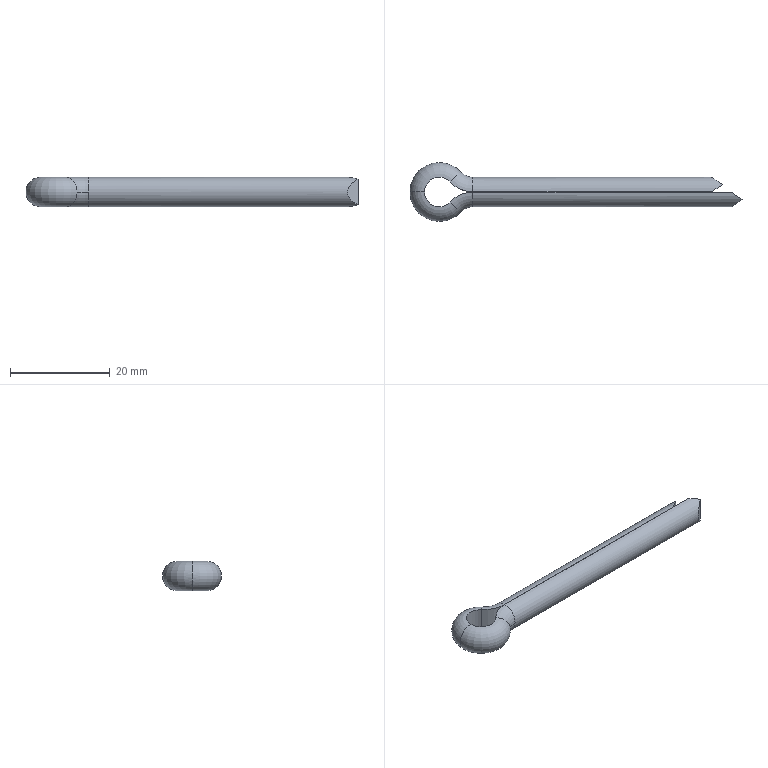Part | SolidWorks | features ICE 1, Sweep 1 | 1 solid | 18 faces | box 66.6 x 11.8 x 5.9 mm | volume 1774 mm3 | torus 6 | cylinder 6 | plane 6 | commonest cylinder face diameters 5.9 x3 12.247 x2 5.92 x1
STEP:
#1=CARTESIAN_POINT('',(6.7,0.01,2.95));
#2=VERTEX_POINT('',#1);
#3=CARTESIAN_POINT('',(6.7,2.95,0.));
#4=VERTEX_POINT('',#3);
#5=CARTESIAN_POINT('',(6.7,0.,0.));
#6=DIRECTION('',(-1.,0.,0.));
#7=DIRECTION('',(0.,0.,1.));
#8=AXIS2_PLACEMENT_3D('',#5,#6,#7);
#9=CIRCLE('',#8,2.95);
#10=EDGE_CURVE('',#2,#4,#9,.T.);
#11=ORIENTED_EDGE('',*,*,#10,.T.);
#12=CARTESIAN_POINT('',(4.352,3.984,0.));
#13=VERTEX_POINT('',#12);
#14=CARTESIAN_POINT('',(6.7,6.133,0.));
#15=DIRECTION('',(0.,0.,-1.));
#16=DIRECTION('',(-1.,0.,0.));
#17=AXIS2_PLACEMENT_3D('',#14,#15,#16);
#18=CIRCLE('',#17,3.183);
#19=EDGE_CURVE('',#4,#13,#18,.T.);
#20=ORIENTED_EDGE('',*,*,#19,.T.);
#21=CARTESIAN_POINT('',(2.183,1.999,2.95));
#22=VERTEX_POINT('',#21);
#23=CARTESIAN_POINT('',(2.176,1.992,0.));
#24=DIRECTION('',(-0.6752,0.7376,0.));
#25=DIRECTION('',(0.,0.,1.));
#26=AXIS2_PLACEMENT_3D('',#23,#24,#25);
#27=CIRCLE('',#26,2.95);
#28=EDGE_CURVE('',#22,#13,#27,.T.);
#29=ORIENTED_EDGE('',*,*,#28,.F.);
#30=CARTESIAN_POINT('',(6.7,6.133,2.95));
#31=DIRECTION('',(0.,0.,-1.));
#32=DIRECTION('',(-1.,0.,0.));
#33=AXIS2_PLACEMENT_3D('',#30,#31,#32);
#34=CIRCLE('',#33,6.123);
#35=EDGE_CURVE('',#2,#22,#34,.T.);
#36=ORIENTED_EDGE('',*,*,#35,.F.);
#37=EDGE_LOOP('',(#11,#20,#29,#36));
#38=FACE_OUTER_BOUND('',#37,.T.);
#39=CARTESIAN_POINT('',(6.7,6.133,0.));
#40=DIRECTION('',(0.,0.,-1.));
#41=DIRECTION('',(-1.,0.,0.));
#42=AXIS2_PLACEMENT_3D('',#39,#40,#41);
#43=TOROIDAL_SURFACE('',#42,6.133,2.95);
#44=ADVANCED_FACE('',(#38),#43,.T.);
#45=CARTESIAN_POINT('',(2.183,-1.999,2.95));
#46=VERTEX_POINT('',#45);
#47=CARTESIAN_POINT('',(4.352,-3.984,0.));
#48=VERTEX_POINT('',#47);
#49=CARTESIAN_POINT('',(2.176,-1.992,0.));
#50=DIRECTION('',(0.6752,0.7376,0.));
#51=DIRECTION('',(0.,0.,1.));
#52=AXIS2_PLACEMENT_3D('',#49,#50,#51);
#53=CIRCLE('',#52,2.95);
#54=EDGE_CURVE('',#46,#48,#53,.T.);
#55=ORIENTED_EDGE('',*,*,#54,.T.);
#56=CARTESIAN_POINT('',(6.7,-2.95,0.));
#57=VERTEX_POINT('',#56);
#58=CARTESIAN_POINT('',(6.7,-6.133,0.));
#59=DIRECTION('',(0.,0.,-1.));
#60=DIRECTION('',(-1.,0.,0.));
#61=AXIS2_PLACEMENT_3D('',#58,#59,#60);
#62=CIRCLE('',#61,3.183);
#63=EDGE_CURVE('',#48,#57,#62,.T.);
#64=ORIENTED_EDGE('',*,*,#63,.T.);
#65=CARTESIAN_POINT('',(6.7,-0.01,2.95));
#66=VERTEX_POINT('',#65);
#67=CARTESIAN_POINT('',(6.7,0.,0.));
#68=DIRECTION('',(1.,0.,0.));
#69=DIRECTION('',(0.,0.,1.));
#70=AXIS2_PLACEMENT_3D('',#67,#68,#69);
#71=CIRCLE('',#70,2.95);
#72=EDGE_CURVE('',#66,#57,#71,.T.);
#73=ORIENTED_EDGE('',*,*,#72,.F.);
#74=CARTESIAN_POINT('',(6.7,-6.133,2.95));
#75=DIRECTION('',(0.,0.,-1.));
#76=DIRECTION('',(-1.,0.,0.));
#77=AXIS2_PLACEMENT_3D('',#74,#75,#76);
#78=CIRCLE('',#77,6.123);
#79=EDGE_CURVE('',#46,#66,#78,.T.);
#80=ORIENTED_EDGE('',*,*,#79,.F.);
#81=EDGE_LOOP('',(#55,#64,#73,#80));
#82=FACE_OUTER_BOUND('',#81,.T.);
#83=CARTESIAN_POINT('',(6.7,-6.133,0.));
#84=DIRECTION('',(0.,0.,-1.));
#85=DIRECTION('',(-1.,0.,0.));
#86=AXIS2_PLACEMENT_3D('',#83,#84,#85);
#87=TOROIDAL_SURFACE('',#86,6.133,2.95);
#88=ADVANCED_FACE('',(#82),#87,.T.);
#89=CARTESIAN_POINT('',(6.7,0.01,-2.95));
#90=VERTEX_POINT('',#89);
#91=CARTESIAN_POINT('',(6.7,0.,0.));
#92=DIRECTION('',(-1.,0.,0.));
#93=DIRECTION('',(0.,0.,1.));
#94=AXIS2_PLACEMENT_3D('',#91,#92,#93);
#95=CIRCLE('',#94,2.95);
#96=EDGE_CURVE('',#4,#90,#95,.T.);
#97=ORIENTED_EDGE('',*,*,#96,.F.);
#98=CARTESIAN_POINT('',(54.597,2.95,0.));
#99=VERTEX_POINT('',#98);
#100=CARTESIAN_POINT('',(6.7,2.95,0.));
#101=DIRECTION('',(1.,0.,0.));
#102=VECTOR('',#101,1000.);
#103=LINE('',#100,#102);
#104=EDGE_CURVE('',#4,#99,#103,.T.);
#105=ORIENTED_EDGE('',*,*,#104,.T.);
#106=CARTESIAN_POINT('',(56.7,1.47,-2.558));
#107=VERTEX_POINT('',#106);
#108=CARTESIAN_POINT('',(54.597,2.95,0.));
#109=CARTESIAN_POINT('',(54.597,2.95,-1.082));
#110=CARTESIAN_POINT('',(55.367,2.408,-2.018));
#111=CARTESIAN_POINT('',(56.7,1.47,-2.558));
#112=(BOUNDED_CURVE()B_SPLINE_CURVE(3,(#108,#109,#110,#111),.UNSPECIFIED.,.F.,.T.)B_SPLINE_CURVE_WITH_KNOTS((4,4),(3.142,4.191),.UNSPECIFIED.)CURVE()GEOMETRIC_REPRESENTATION_ITEM()RATIONAL_B_SPLINE_CURVE((1.,0.9104,0.9104,1.))REPRESENTATION_ITEM(''));
#113=EDGE_CURVE('',#99,#107,#112,.T.);
#114=ORIENTED_EDGE('',*,*,#113,.T.);
#115=CARTESIAN_POINT('',(54.604,0.01,-2.95));
#116=VERTEX_POINT('',#115);
#117=CARTESIAN_POINT('',(56.7,1.47,-2.558));
#118=CARTESIAN_POINT('',(56.059,1.023,-2.814));
#119=CARTESIAN_POINT('',(55.344,0.5254,-2.948));
#120=CARTESIAN_POINT('',(54.604,0.01,-2.95));
#121=(BOUNDED_CURVE()B_SPLINE_CURVE(3,(#117,#118,#119,#120),.UNSPECIFIED.,.F.,.T.)B_SPLINE_CURVE_WITH_KNOTS((4,4),(1.049,1.567),.UNSPECIFIED.)CURVE()GEOMETRIC_REPRESENTATION_ITEM()RATIONAL_B_SPLINE_CURVE((1.,0.9777,0.9777,1.))REPRESENTATION_ITEM(''));
#122=EDGE_CURVE('',#107,#116,#121,.T.);
#123=ORIENTED_EDGE('',*,*,#122,.T.);
#124=CARTESIAN_POINT('',(6.7,0.01,-2.95));
#125=DIRECTION('',(1.,0.,0.));
#126=VECTOR('',#125,1000.);
#127=LINE('',#124,#126);
#128=EDGE_CURVE('',#90,#116,#127,.T.);
#129=ORIENTED_EDGE('',*,*,#128,.F.);
#130=EDGE_LOOP('',(#97,#105,#114,#123,#129));
#131=FACE_OUTER_BOUND('',#130,.T.);
#132=CARTESIAN_POINT('',(6.7,0.,0.));
#133=DIRECTION('',(1.,0.,0.));
#134=DIRECTION('',(0.,1.,0.));
#135=AXIS2_PLACEMENT_3D('',#132,#133,#134);
#136=CYLINDRICAL_SURFACE('',#135,2.95);
#137=ADVANCED_FACE('',(#131),#136,.T.);
#138=CARTESIAN_POINT('',(2.183,1.999,-2.95));
#139=VERTEX_POINT('',#138);
#140=CARTESIAN_POINT('',(-2.96,0.,-2.95));
#141=VERTEX_POINT('',#140);
#142=CARTESIAN_POINT('',(0.,0.,-2.95));
#143=DIRECTION('',(0.,0.,1.));
#144=DIRECTION('',(1.,0.,0.));
#145=AXIS2_PLACEMENT_3D('',#142,#143,#144);
#146=CIRCLE('',#145,2.96);
#147=EDGE_CURVE('',#139,#141,#146,.T.);
#148=ORIENTED_EDGE('',*,*,#147,.T.);
#149=CARTESIAN_POINT('',(-2.96,0.,2.95));
#150=VERTEX_POINT('',#149);
#151=CARTESIAN_POINT('',(-2.95,0.,0.));
#152=DIRECTION('',(0.,1.,0.));
#153=DIRECTION('',(-1.,0.,0.));
#154=AXIS2_PLACEMENT_3D('',#151,#152,#153);
#155=CIRCLE('',#154,2.95);
#156=EDGE_CURVE('',#141,#150,#155,.T.);
#157=ORIENTED_EDGE('',*,*,#156,.T.);
#158=CARTESIAN_POINT('',(0.,0.,2.95));
#159=DIRECTION('',(0.,0.,1.));
#160=DIRECTION('',(1.,0.,0.));
#161=AXIS2_PLACEMENT_3D('',#158,#159,#160);
#162=CIRCLE('',#161,2.96);
#163=EDGE_CURVE('',#22,#150,#162,.T.);
#164=ORIENTED_EDGE('',*,*,#163,.F.);
#165=ORIENTED_EDGE('',*,*,#28,.T.);
#166=CARTESIAN_POINT('',(2.176,1.992,0.));
#167=DIRECTION('',(-0.6752,0.7376,0.));
#168=DIRECTION('',(0.,0.,1.));
#169=AXIS2_PLACEMENT_3D('',#166,#167,#168);
#170=CIRCLE('',#169,2.95);
#171=EDGE_CURVE('',#13,#139,#170,.T.);
#172=ORIENTED_EDGE('',*,*,#171,.T.);
#173=EDGE_LOOP('',(#148,#157,#164,#165,#172));
#174=FACE_OUTER_BOUND('',#173,.T.);
#175=CARTESIAN_POINT('',(0.,0.,0.));
#176=DIRECTION('',(0.,0.,1.));
#177=DIRECTION('',(1.,0.,0.));
#178=AXIS2_PLACEMENT_3D('',#175,#176,#177);
#179=TOROIDAL_SURFACE('',#178,2.95,2.95);
#180=ADVANCED_FACE('',(#174),#179,.T.);
#181=CARTESIAN_POINT('',(60.7,-1.48,-2.552));
#182=VERTEX_POINT('',#181);
#183=CARTESIAN_POINT('',(58.611,-0.01,-2.95));
#184=VERTEX_POINT('',#183);
#185=CARTESIAN_POINT('',(60.7,-1.48,-2.552));
#186=CARTESIAN_POINT('',(60.062,-1.031,-2.812));
#187=CARTESIAN_POINT('',(59.349,-0.5294,-2.948));
#188=CARTESIAN_POINT('',(58.611,-0.01,-2.95));
#189=(BOUNDED_CURVE()B_SPLINE_CURVE(3,(#185,#186,#187,#188),.UNSPECIFIED.,.F.,.F.)B_SPLINE_CURVE_WITH_KNOTS((4,4),(1.045,1.567),.UNSPECIFIED.)CURVE()GEOMETRIC_REPRESENTATION_ITEM()RATIONAL_B_SPLINE_CURVE((1.,0.9774,0.9774,1.))REPRESENTATION_ITEM(''));
#190=EDGE_CURVE('',#182,#184,#189,.T.);
#191=ORIENTED_EDGE('',*,*,#190,.F.);
#192=CARTESIAN_POINT('',(60.7,-1.48,2.552));
#193=VERTEX_POINT('',#192);
#194=CARTESIAN_POINT('',(60.7,-1.48,2.552));
#195=CARTESIAN_POINT('',(57.537,-3.684,1.274));
#196=CARTESIAN_POINT('',(57.537,-3.684,-1.274));
#197=CARTESIAN_POINT('',(60.7,-1.48,-2.552));
#198=(BOUNDED_CURVE()B_SPLINE_CURVE(3,(#194,#195,#196,#197),.UNSPECIFIED.,.F.,.T.)B_SPLINE_CURVE_WITH_KNOTS((4,4),(2.096,4.187),.UNSPECIFIED.)CURVE()GEOMETRIC_REPRESENTATION_ITEM()RATIONAL_B_SPLINE_CURVE((1.,0.6678,0.6678,1.))REPRESENTATION_ITEM(''));
#199=EDGE_CURVE('',#193,#182,#198,.T.);
#200=ORIENTED_EDGE('',*,*,#199,.F.);
#201=CARTESIAN_POINT('',(58.611,-0.01,2.95));
#202=VERTEX_POINT('',#201);
#203=CARTESIAN_POINT('',(58.611,-0.01,2.95));
#204=CARTESIAN_POINT('',(59.349,-0.5294,2.948));
#205=CARTESIAN_POINT('',(60.062,-1.031,2.812));
#206=CARTESIAN_POINT('',(60.7,-1.48,2.552));
#207=(BOUNDED_CURVE()B_SPLINE_CURVE(3,(#203,#204,#205,#206),.UNSPECIFIED.,.F.,.F.)B_SPLINE_CURVE_WITH_KNOTS((4,4),(4.716,5.238),.UNSPECIFIED.)CURVE()GEOMETRIC_REPRESENTATION_ITEM()RATIONAL_B_SPLINE_CURVE((1.,0.9774,0.9774,1.))REPRESENTATION_ITEM(''));
#208=EDGE_CURVE('',#202,#193,#207,.T.);
#209=ORIENTED_EDGE('',*,*,#208,.F.);
#210=CARTESIAN_POINT('',(6.7,-0.01,2.95));
#211=DIRECTION('',(1.,0.,0.));
#212=VECTOR('',#211,1000.);
#213=LINE('',#210,#212);
#214=EDGE_CURVE('',#66,#202,#213,.T.);
#215=ORIENTED_EDGE('',*,*,#214,.F.);
#216=ORIENTED_EDGE('',*,*,#72,.T.);
#217=CARTESIAN_POINT('',(6.7,-0.01,-2.95));
#218=VERTEX_POINT('',#217);
#219=CARTESIAN_POINT('',(6.7,0.,0.));
#220=DIRECTION('',(1.,0.,0.));
#221=DIRECTION('',(0.,0.,1.));
#222=AXIS2_PLACEMENT_3D('',#219,#220,#221);
#223=CIRCLE('',#222,2.95);
#224=EDGE_CURVE('',#57,#218,#223,.T.);
#225=ORIENTED_EDGE('',*,*,#224,.T.);
#226=CARTESIAN_POINT('',(6.7,-0.01,-2.95));
#227=DIRECTION('',(1.,0.,0.));
#228=VECTOR('',#227,1000.);
#229=LINE('',#226,#228);
#230=EDGE_CURVE('',#218,#184,#229,.T.);
#231=ORIENTED_EDGE('',*,*,#230,.T.);
#232=EDGE_LOOP('',(#191,#200,#209,#215,#216,#225,#231));
#233=FACE_OUTER_BOUND('',#232,.T.);
#234=CARTESIAN_POINT('',(6.7,0.,0.));
#235=DIRECTION('',(1.,0.,0.));
#236=DIRECTION('',(0.,1.,0.));
#237=AXIS2_PLACEMENT_3D('',#234,#235,#236);
#238=CYLINDRICAL_SURFACE('',#237,2.95);
#239=ADVANCED_FACE('',(#233),#238,.T.);
#240=CARTESIAN_POINT('',(58.611,-0.01,-2.95));
#241=DIRECTION('',(0.,0.,1.));
#242=VECTOR('',#241,1000.);
#243=LINE('',#240,#242);
#244=EDGE_CURVE('',#184,#202,#243,.T.);
#245=ORIENTED_EDGE('',*,*,#244,.F.);
#246=ORIENTED_EDGE('',*,*,#230,.F.);
#247=CARTESIAN_POINT('',(6.7,-0.01,-2.95));
#248=DIRECTION('',(0.,0.,1.));
#249=VECTOR('',#248,1000.);
#250=LINE('',#247,#249);
#251=EDGE_CURVE('',#218,#66,#250,.T.);
#252=ORIENTED_EDGE('',*,*,#251,.T.);
#253=ORIENTED_EDGE('',*,*,#214,.T.);
#254=EDGE_LOOP('',(#245,#246,#252,#253));
#255=FACE_OUTER_BOUND('',#254,.T.);
#256=CARTESIAN_POINT('',(6.7,-0.01,-2.95));
#257=DIRECTION('',(0.,1.,0.));
#258=DIRECTION('',(-1.,0.,0.));
#259=AXIS2_PLACEMENT_3D('',#256,#257,#258);
#260=PLANE('',#259);
#261=ADVANCED_FACE('',(#255),#260,.T.);
#262=CARTESIAN_POINT('',(2.183,-1.999,-2.95));
#263=VERTEX_POINT('',#262);
#264=CARTESIAN_POINT('',(2.183,-1.999,-2.95));
#265=DIRECTION('',(0.,0.,1.));
#266=VECTOR('',#265,1000.);
#267=LINE('',#264,#266);
#268=EDGE_CURVE('',#263,#46,#267,.T.);
#269=ORIENTED_EDGE('',*,*,#268,.T.);
#270=ORIENTED_EDGE('',*,*,#79,.T.);
#271=ORIENTED_EDGE('',*,*,#251,.F.);
#272=CARTESIAN_POINT('',(6.7,-6.133,-2.95));
#273=DIRECTION('',(0.,0.,-1.));
#274=DIRECTION('',(-1.,0.,0.));
#275=AXIS2_PLACEMENT_3D('',#272,#273,#274);
#276=CIRCLE('',#275,6.123);
#277=EDGE_CURVE('',#263,#218,#276,.T.);
#278=ORIENTED_EDGE('',*,*,#277,.F.);
#279=EDGE_LOOP('',(#269,#270,#271,#278));
#280=FACE_OUTER_BOUND('',#279,.T.);
#281=CARTESIAN_POINT('',(6.7,-6.133,0.));
#282=DIRECTION('',(0.,0.,-1.));
#283=DIRECTION('',(-1.,0.,0.));
#284=AXIS2_PLACEMENT_3D('',#281,#282,#283);
#285=CYLINDRICAL_SURFACE('',#284,6.123);
#286=ADVANCED_FACE('',(#280),#285,.T.);
#287=ORIENTED_EDGE('',*,*,#63,.F.);
#288=CARTESIAN_POINT('',(2.176,-1.992,0.));
#289=DIRECTION('',(0.6752,0.7376,0.));
#290=DIRECTION('',(0.,0.,1.));
#291=AXIS2_PLACEMENT_3D('',#288,#289,#290);
#292=CIRCLE('',#291,2.95);
#293=EDGE_CURVE('',#48,#263,#292,.T.);
#294=ORIENTED_EDGE('',*,*,#293,.T.);
#295=ORIENTED_EDGE('',*,*,#277,.T.);
#296=ORIENTED_EDGE('',*,*,#224,.F.);
#297=EDGE_LOOP('',(#287,#294,#295,#296));
#298=FACE_OUTER_BOUND('',#297,.T.);
#299=CARTESIAN_POINT('',(6.7,-6.133,0.));
#300=DIRECTION('',(0.,0.,-1.));
#301=DIRECTION('',(-1.,0.,0.));
#302=AXIS2_PLACEMENT_3D('',#299,#300,#301);
#303=TOROIDAL_SURFACE('',#302,6.133,2.95);
#304=ADVANCED_FACE('',(#298),#303,.T.);
#305=CARTESIAN_POINT('',(2.183,1.999,-2.95));
#306=DIRECTION('',(0.,0.,1.));
#307=VECTOR('',#306,1000.);
#308=LINE('',#305,#307);
#309=EDGE_CURVE('',#139,#22,#308,.T.);
#310=ORIENTED_EDGE('',*,*,#309,.T.);
#311=ORIENTED_EDGE('',*,*,#163,.T.);
#312=CARTESIAN_POINT('',(0.,0.,2.95));
#313=DIRECTION('',(0.,0.,1.));
#314=DIRECTION('',(1.,0.,0.));
#315=AXIS2_PLACEMENT_3D('',#312,#313,#314);
#316=CIRCLE('',#315,2.96);
#317=EDGE_CURVE('',#150,#46,#316,.T.);
#318=ORIENTED_EDGE('',*,*,#317,.T.);
#319=ORIENTED_EDGE('',*,*,#268,.F.);
#320=CARTESIAN_POINT('',(0.,0.,-2.95));
#321=DIRECTION('',(0.,0.,1.));
#322=DIRECTION('',(1.,0.,0.));
#323=AXIS2_PLACEMENT_3D('',#320,#321,#322);
#324=CIRCLE('',#323,2.96);
#325=EDGE_CURVE('',#141,#263,#324,.T.);
#326=ORIENTED_EDGE('',*,*,#325,.F.);
#327=ORIENTED_EDGE('',*,*,#147,.F.);
#328=EDGE_LOOP('',(#310,#311,#318,#319,#326,#327));
#329=FACE_OUTER_BOUND('',#328,.T.);
#330=CARTESIAN_POINT('',(0.,0.,0.));
#331=DIRECTION('',(0.,0.,1.));
#332=DIRECTION('',(1.,0.,0.));
#333=AXIS2_PLACEMENT_3D('',#330,#331,#332);
#334=CYLINDRICAL_SURFACE('',#333,2.96);
#335=ADVANCED_FACE('',(#329),#334,.F.);
#336=ORIENTED_EDGE('',*,*,#156,.F.);
#337=ORIENTED_EDGE('',*,*,#325,.T.);
#338=ORIENTED_EDGE('',*,*,#293,.F.);
#339=ORIENTED_EDGE('',*,*,#54,.F.);
#340=ORIENTED_EDGE('',*,*,#317,.F.);
#341=EDGE_LOOP('',(#336,#337,#338,#339,#340));
#342=FACE_OUTER_BOUND('',#341,.T.);
#343=CARTESIAN_POINT('',(0.,0.,0.));
#344=DIRECTION('',(0.,0.,1.));
#345=DIRECTION('',(1.,0.,0.));
#346=AXIS2_PLACEMENT_3D('',#343,#344,#345);
#347=TOROIDAL_SURFACE('',#346,2.95,2.95);
#348=ADVANCED_FACE('',(#342),#347,.T.);
#349=CARTESIAN_POINT('',(6.7,0.01,-2.95));
#350=DIRECTION('',(0.,0.,1.));
#351=VECTOR('',#350,1000.);
#352=LINE('',#349,#351);
#353=EDGE_CURVE('',#90,#2,#352,.T.);
#354=ORIENTED_EDGE('',*,*,#353,.T.);
#355=ORIENTED_EDGE('',*,*,#35,.T.);
#356=ORIENTED_EDGE('',*,*,#309,.F.);
#357=CARTESIAN_POINT('',(6.7,6.133,-2.95));
#358=DIRECTION('',(0.,0.,-1.));
#359=DIRECTION('',(-1.,0.,0.));
#360=AXIS2_PLACEMENT_3D('',#357,#358,#359);
#361=CIRCLE('',#360,6.123);
#362=EDGE_CURVE('',#90,#139,#361,.T.);
#363=ORIENTED_EDGE('',*,*,#362,.F.);
#364=EDGE_LOOP('',(#354,#355,#356,#363));
#365=FACE_OUTER_BOUND('',#364,.T.);
#366=CARTESIAN_POINT('',(6.7,6.133,0.));
#367=DIRECTION('',(0.,0.,-1.));
#368=DIRECTION('',(-1.,0.,0.));
#369=AXIS2_PLACEMENT_3D('',#366,#367,#368);
#370=CYLINDRICAL_SURFACE('',#369,6.123);
#371=ADVANCED_FACE('',(#365),#370,.T.);
#372=ORIENTED_EDGE('',*,*,#19,.F.);
#373=ORIENTED_EDGE('',*,*,#96,.T.);
#374=ORIENTED_EDGE('',*,*,#362,.T.);
#375=ORIENTED_EDGE('',*,*,#171,.F.);
#376=EDGE_LOOP('',(#372,#373,#374,#375));
#377=FACE_OUTER_BOUND('',#376,.T.);
#378=CARTESIAN_POINT('',(6.7,6.133,0.));
#379=DIRECTION('',(0.,0.,-1.));
#380=DIRECTION('',(-1.,0.,0.));
#381=AXIS2_PLACEMENT_3D('',#378,#379,#380);
#382=TOROIDAL_SURFACE('',#381,6.133,2.95);
#383=ADVANCED_FACE('',(#377),#382,.T.);
#384=ORIENTED_EDGE('',*,*,#104,.F.);
#385=ORIENTED_EDGE('',*,*,#10,.F.);
#386=CARTESIAN_POINT('',(54.604,0.01,2.95));
#387=VERTEX_POINT('',#386);
#388=CARTESIAN_POINT('',(6.7,0.01,2.95));
#389=DIRECTION('',(1.,0.,0.));
#390=VECTOR('',#389,1000.);
#391=LINE('',#388,#390);
#392=EDGE_CURVE('',#2,#387,#391,.T.);
#393=ORIENTED_EDGE('',*,*,#392,.T.);
#394=CARTESIAN_POINT('',(56.7,1.47,2.558));
#395=VERTEX_POINT('',#394);
#396=CARTESIAN_POINT('',(54.604,0.01,2.95));
#397=CARTESIAN_POINT('',(55.344,0.5254,2.948));
#398=CARTESIAN_POINT('',(56.059,1.023,2.814));
#399=CARTESIAN_POINT('',(56.7,1.47,2.558));
#400=(BOUNDED_CURVE()B_SPLINE_CURVE(3,(#396,#397,#398,#399),.UNSPECIFIED.,.F.,.F.)B_SPLINE_CURVE_WITH_KNOTS((4,4),(4.716,5.234),.UNSPECIFIED.)CURVE()GEOMETRIC_REPRESENTATION_ITEM()RATIONAL_B_SPLINE_CURVE((1.,0.9777,0.9777,1.))REPRESENTATION_ITEM(''));
#401=EDGE_CURVE('',#387,#395,#400,.T.);
#402=ORIENTED_EDGE('',*,*,#401,.T.);
#403=CARTESIAN_POINT('',(56.7,1.47,2.558));
#404=CARTESIAN_POINT('',(55.367,2.408,2.018));
#405=CARTESIAN_POINT('',(54.597,2.95,1.082));
#406=CARTESIAN_POINT('',(54.597,2.95,0.));
#407=(BOUNDED_CURVE()B_SPLINE_CURVE(3,(#403,#404,#405,#406),.UNSPECIFIED.,.F.,.F.)B_SPLINE_CURVE_WITH_KNOTS((4,4),(2.092,3.142),.UNSPECIFIED.)CURVE()GEOMETRIC_REPRESENTATION_ITEM()RATIONAL_B_SPLINE_CURVE((1.,0.9104,0.9104,1.))REPRESENTATION_ITEM(''));
#408=EDGE_CURVE('',#395,#99,#407,.T.);
#409=ORIENTED_EDGE('',*,*,#408,.T.);
#410=EDGE_LOOP('',(#384,#385,#393,#402,#409));
#411=FACE_OUTER_BOUND('',#410,.T.);
#412=CARTESIAN_POINT('',(6.7,0.,0.));
#413=DIRECTION('',(1.,0.,0.));
#414=DIRECTION('',(0.,1.,0.));
#415=AXIS2_PLACEMENT_3D('',#412,#413,#414);
#416=CYLINDRICAL_SURFACE('',#415,2.95);
#417=ADVANCED_FACE('',(#411),#416,.T.);
#418=ORIENTED_EDGE('',*,*,#128,.T.);
#419=CARTESIAN_POINT('',(54.604,0.01,-2.95));
#420=DIRECTION('',(0.,0.,1.));
#421=VECTOR('',#420,1000.);
#422=LINE('',#419,#421);
#423=EDGE_CURVE('',#116,#387,#422,.T.);
#424=ORIENTED_EDGE('',*,*,#423,.T.);
#425=ORIENTED_EDGE('',*,*,#392,.F.);
#426=ORIENTED_EDGE('',*,*,#353,.F.);
#427=EDGE_LOOP('',(#418,#424,#425,#426));
#428=FACE_OUTER_BOUND('',#427,.T.);
#429=CARTESIAN_POINT('',(6.7,0.01,-2.95));
#430=DIRECTION('',(0.,1.,0.));
#431=DIRECTION('',(-1.,0.,0.));
#432=AXIS2_PLACEMENT_3D('',#429,#430,#431);
#433=PLANE('',#432);
#434=ADVANCED_FACE('',(#428),#433,.F.);
#435=CARTESIAN_POINT('',(56.7,1.47,-2.95));
#436=DIRECTION('',(0.,0.,1.));
#437=VECTOR('',#436,1000.);
#438=LINE('',#435,#437);
#439=EDGE_CURVE('',#107,#395,#438,.T.);
#440=ORIENTED_EDGE('',*,*,#439,.T.);
#441=ORIENTED_EDGE('',*,*,#401,.F.);
#442=ORIENTED_EDGE('',*,*,#423,.F.);
#443=ORIENTED_EDGE('',*,*,#122,.F.);
#444=EDGE_LOOP('',(#440,#441,#442,#443));
#445=FACE_OUTER_BOUND('',#444,.T.);
#446=CARTESIAN_POINT('',(56.7,1.47,-2.95));
#447=DIRECTION('',(-0.5716,0.8205,0.));
#448=DIRECTION('',(-0.8205,-0.5716,0.));
#449=AXIS2_PLACEMENT_3D('',#446,#447,#448);
#450=PLANE('',#449);
#451=ADVANCED_FACE('',(#445),#450,.F.);
#452=ORIENTED_EDGE('',*,*,#439,.F.);
#453=ORIENTED_EDGE('',*,*,#113,.F.);
#454=ORIENTED_EDGE('',*,*,#408,.F.);
#455=EDGE_LOOP('',(#452,#453,#454));
#456=FACE_OUTER_BOUND('',#455,.T.);
#457=CARTESIAN_POINT('',(56.7,1.47,-2.95));
#458=DIRECTION('',(-0.5755,-0.8178,0.));
#459=DIRECTION('',(0.8178,-0.5755,0.));
#460=AXIS2_PLACEMENT_3D('',#457,#458,#459);
#461=PLANE('',#460);
#462=ADVANCED_FACE('',(#456),#461,.F.);
#463=ORIENTED_EDGE('',*,*,#199,.T.);
#464=CARTESIAN_POINT('',(60.7,-1.48,-2.95));
#465=DIRECTION('',(0.,0.,1.));
#466=VECTOR('',#465,1000.);
#467=LINE('',#464,#466);
#468=EDGE_CURVE('',#182,#193,#467,.T.);
#469=ORIENTED_EDGE('',*,*,#468,.T.);
#470=EDGE_LOOP('',(#463,#469));
#471=FACE_OUTER_BOUND('',#470,.T.);
#472=CARTESIAN_POINT('',(60.7,-1.48,-2.95));
#473=DIRECTION('',(-0.5716,0.8205,0.));
#474=DIRECTION('',(-0.8205,-0.5716,0.));
#475=AXIS2_PLACEMENT_3D('',#472,#473,#474);
#476=PLANE('',#475);
#477=ADVANCED_FACE('',(#471),#476,.F.);
#478=ORIENTED_EDGE('',*,*,#190,.T.);
#479=ORIENTED_EDGE('',*,*,#244,.T.);
#480=ORIENTED_EDGE('',*,*,#208,.T.);
#481=ORIENTED_EDGE('',*,*,#468,.F.);
#482=EDGE_LOOP('',(#478,#479,#480,#481));
#483=FACE_OUTER_BOUND('',#482,.T.);
#484=CARTESIAN_POINT('',(60.7,-1.48,-2.95));
#485=DIRECTION('',(-0.5755,-0.8178,0.));
#486=DIRECTION('',(0.8178,-0.5755,0.));
#487=AXIS2_PLACEMENT_3D('',#484,#485,#486);
#488=PLANE('',#487);
#489=ADVANCED_FACE('',(#483),#488,.F.);
#490=CLOSED_SHELL('',(#44,#88,#137,#180,#239,#261,#286,#304,#335,#348,#371,#383,#417,#434,#451,#462,#477,#489));
#491=MANIFOLD_SOLID_BREP('',#490);
#492=CARTESIAN_POINT('',(0.,0.,0.));
#493=DIRECTION('',(0.,0.,1.));
#494=DIRECTION('',(1.,0.,0.));
#495=AXIS2_PLACEMENT_3D('',#492,#493,#494);
#496=(LENGTH_UNIT()NAMED_UNIT(*)SI_UNIT(.MILLI.,.METRE.));
#497=UNCERTAINTY_MEASURE_WITH_UNIT(LENGTH_MEASURE(0.00001),#496,'','');
#498=(NAMED_UNIT(*)PLANE_ANGLE_UNIT()SI_UNIT($,.RADIAN.));
#499=(NAMED_UNIT(*)SI_UNIT($,.STERADIAN.)SOLID_ANGLE_UNIT());
#500=(GEOMETRIC_REPRESENTATION_CONTEXT(3)GLOBAL_UNCERTAINTY_ASSIGNED_CONTEXT((#497))GLOBAL_UNIT_ASSIGNED_CONTEXT((#496,#498,#499))REPRESENTATION_CONTEXT('',''));
#501=ADVANCED_BREP_SHAPE_REPRESENTATION('',(#491,#495),#500);